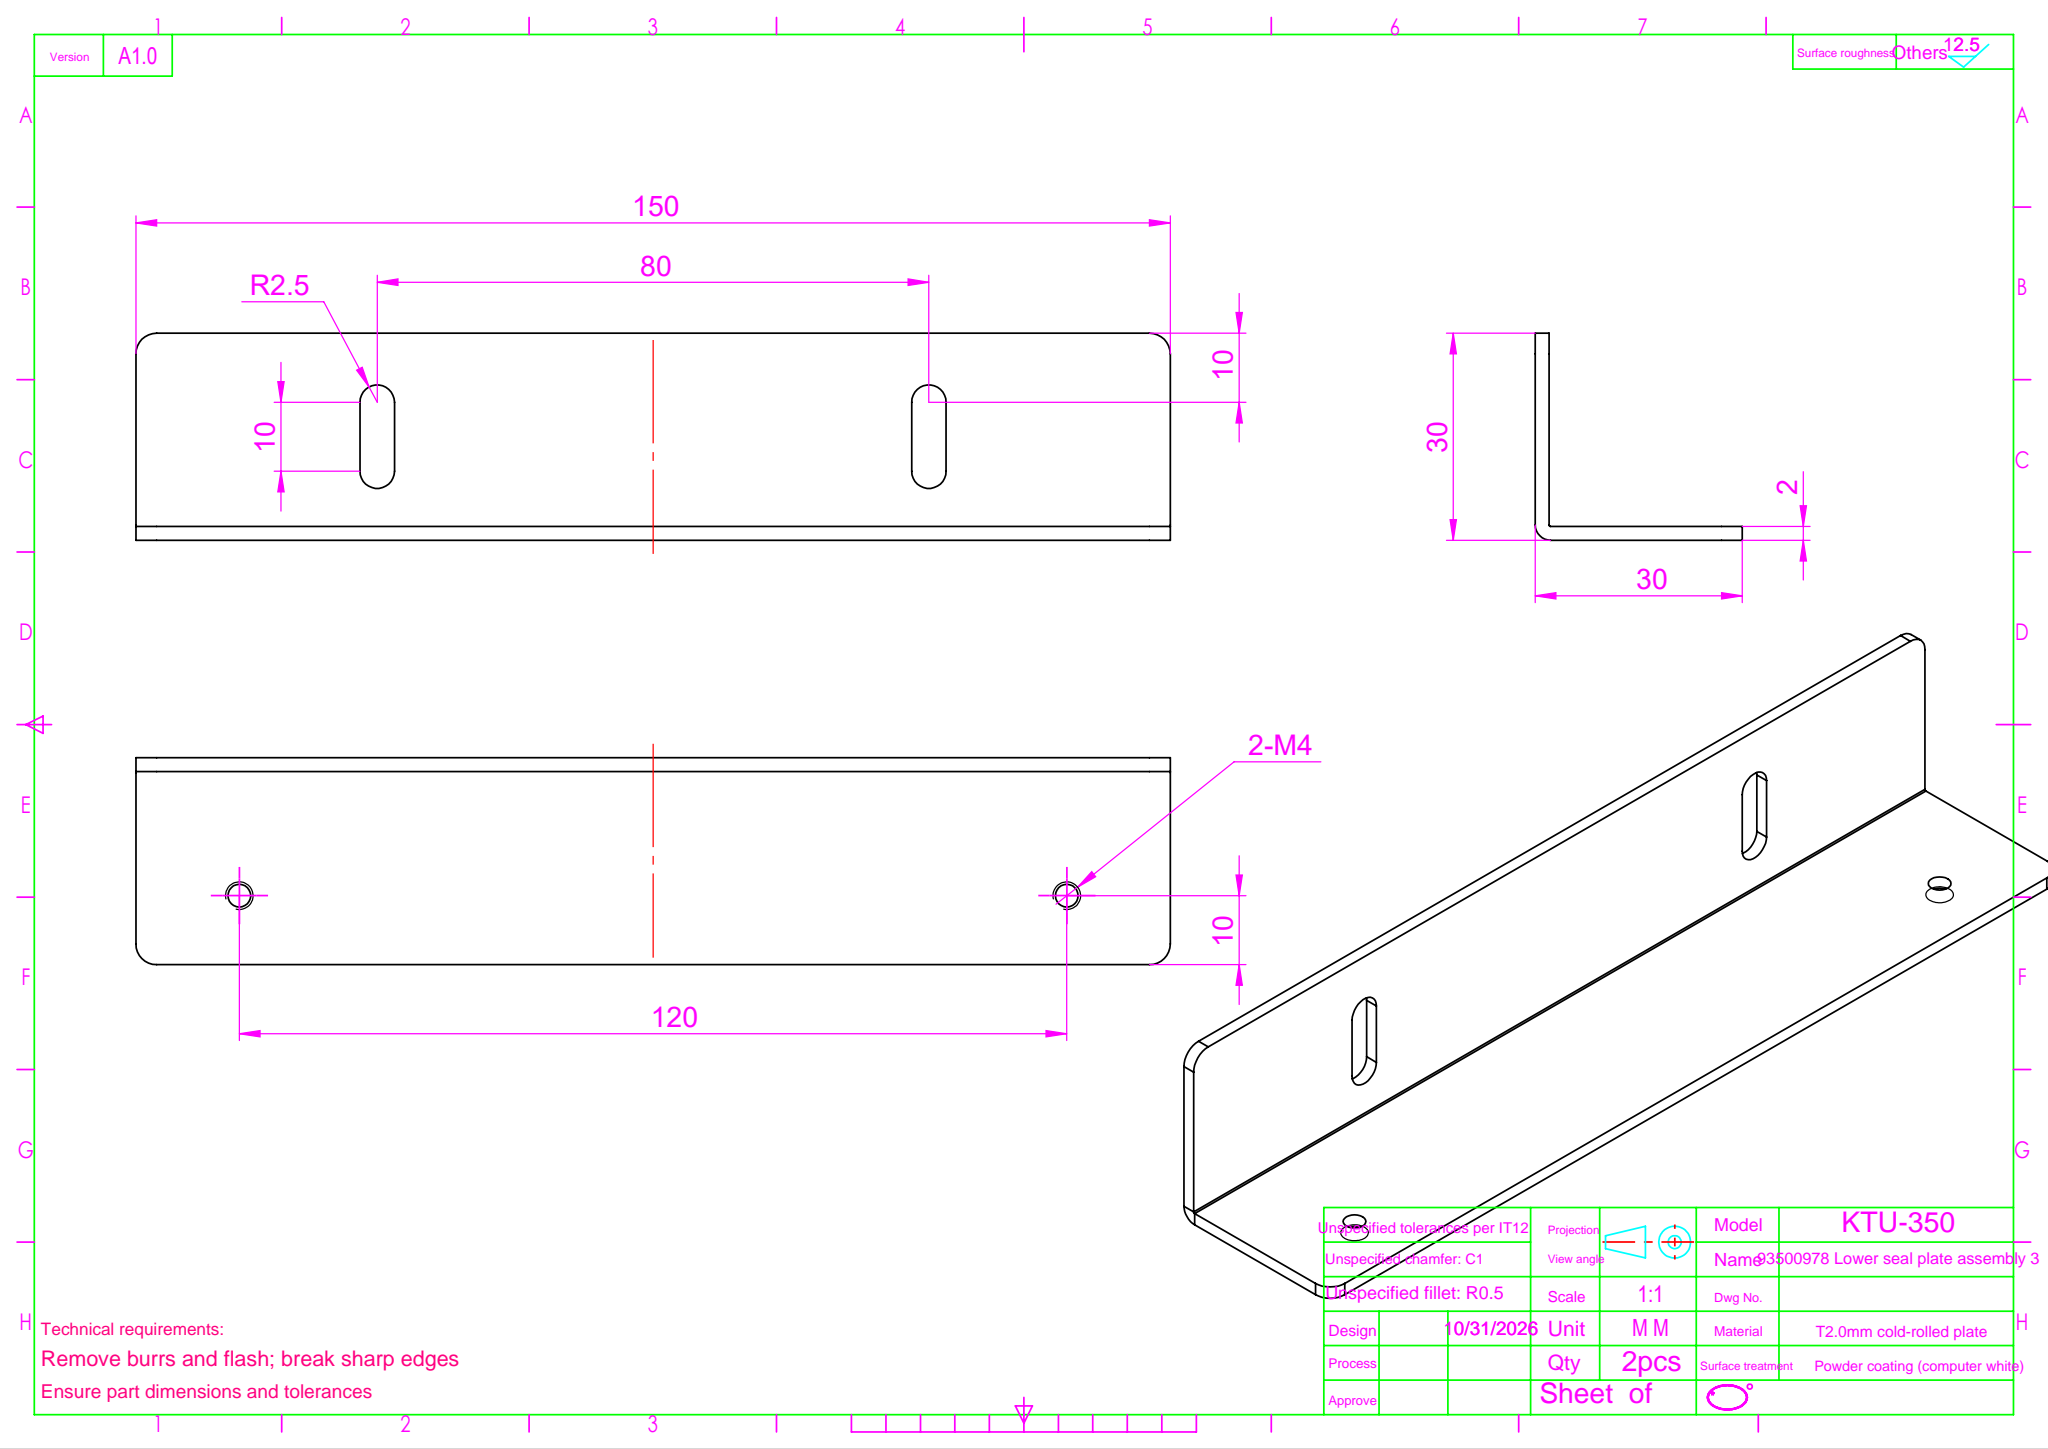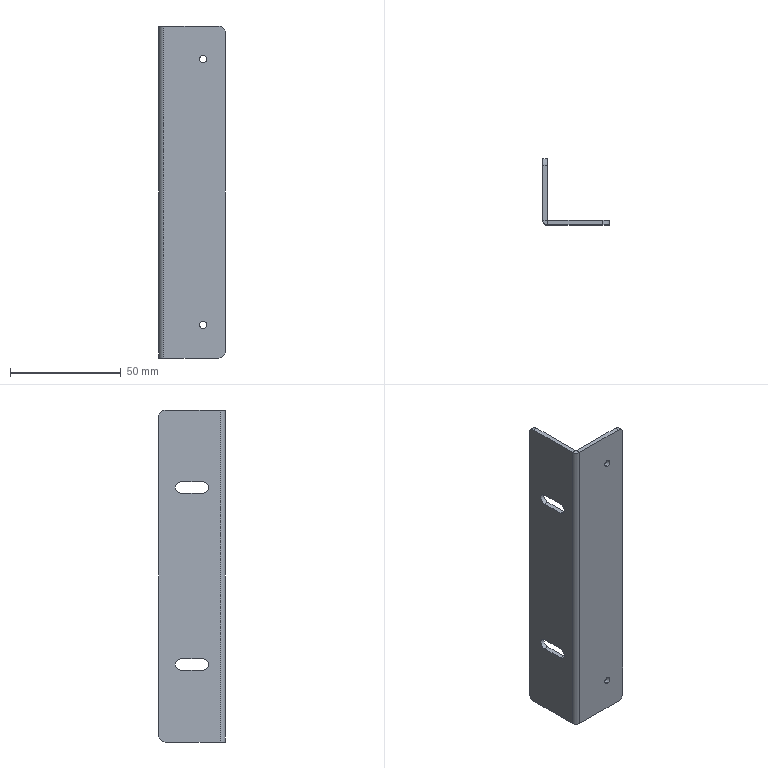Part | SolidWorks | features Fillet 1, FlatPattern 1, HoleWzd 1, ICE 1, SMBaseFlange 1, SheetMetal 1 | 1 solid | 32 faces | box 30 x 30 x 150 mm | volume 16917 mm3 | cylinder 16 | plane 16 | commonest cylinder face diameters 5 x6 3.3 x4 6 x4 0.4 x1 4.4 x1
STEP:
#1=CARTESIAN_POINT('',(5.,2.,61.65));
#2=VERTEX_POINT('',#1);
#3=CARTESIAN_POINT('',(5.,2.,58.35));
#4=VERTEX_POINT('',#3);
#5=CARTESIAN_POINT('',(5.,2.,60.));
#6=DIRECTION('',(0.,-1.,0.));
#7=DIRECTION('',(0.,0.,-1.));
#8=AXIS2_PLACEMENT_3D('',#5,#6,#7);
#9=CIRCLE('',#8,1.65);
#10=EDGE_CURVE('',#2,#4,#9,.T.);
#11=ORIENTED_EDGE('',*,*,#10,.F.);
#12=CARTESIAN_POINT('',(5.,0.,61.65));
#13=VERTEX_POINT('',#12);
#14=CARTESIAN_POINT('',(5.,0.,61.65));
#15=DIRECTION('',(0.,-1.,0.));
#16=VECTOR('',#15,1000.);
#17=LINE('',#14,#16);
#18=EDGE_CURVE('',#2,#13,#17,.T.);
#19=ORIENTED_EDGE('',*,*,#18,.T.);
#20=CARTESIAN_POINT('',(5.,0.,58.35));
#21=VERTEX_POINT('',#20);
#22=CARTESIAN_POINT('',(5.,0.,60.));
#23=DIRECTION('',(0.,-1.,0.));
#24=DIRECTION('',(0.,0.,-1.));
#25=AXIS2_PLACEMENT_3D('',#22,#23,#24);
#26=CIRCLE('',#25,1.65);
#27=EDGE_CURVE('',#13,#21,#26,.T.);
#28=ORIENTED_EDGE('',*,*,#27,.T.);
#29=CARTESIAN_POINT('',(5.,0.,58.35));
#30=DIRECTION('',(0.,-1.,0.));
#31=VECTOR('',#30,1000.);
#32=LINE('',#29,#31);
#33=EDGE_CURVE('',#4,#21,#32,.T.);
#34=ORIENTED_EDGE('',*,*,#33,.F.);
#35=EDGE_LOOP('',(#11,#19,#28,#34));
#36=FACE_OUTER_BOUND('',#35,.T.);
#37=CARTESIAN_POINT('',(5.,0.,60.));
#38=DIRECTION('',(0.,-1.,0.));
#39=DIRECTION('',(0.,0.,-1.));
#40=AXIS2_PLACEMENT_3D('',#37,#38,#39);
#41=CYLINDRICAL_SURFACE('',#40,1.65);
#42=ADVANCED_FACE('',(#36),#41,.F.);
#43=CARTESIAN_POINT('',(5.,2.,-58.35));
#44=VERTEX_POINT('',#43);
#45=CARTESIAN_POINT('',(5.,2.,-61.65));
#46=VERTEX_POINT('',#45);
#47=CARTESIAN_POINT('',(5.,2.,-60.));
#48=DIRECTION('',(0.,-1.,0.));
#49=DIRECTION('',(0.,0.,-1.));
#50=AXIS2_PLACEMENT_3D('',#47,#48,#49);
#51=CIRCLE('',#50,1.65);
#52=EDGE_CURVE('',#44,#46,#51,.T.);
#53=ORIENTED_EDGE('',*,*,#52,.F.);
#54=CARTESIAN_POINT('',(5.,0.,-58.35));
#55=VERTEX_POINT('',#54);
#56=CARTESIAN_POINT('',(5.,0.,-58.35));
#57=DIRECTION('',(0.,-1.,0.));
#58=VECTOR('',#57,1000.);
#59=LINE('',#56,#58);
#60=EDGE_CURVE('',#44,#55,#59,.T.);
#61=ORIENTED_EDGE('',*,*,#60,.T.);
#62=CARTESIAN_POINT('',(5.,0.,-61.65));
#63=VERTEX_POINT('',#62);
#64=CARTESIAN_POINT('',(5.,0.,-60.));
#65=DIRECTION('',(0.,-1.,0.));
#66=DIRECTION('',(0.,0.,-1.));
#67=AXIS2_PLACEMENT_3D('',#64,#65,#66);
#68=CIRCLE('',#67,1.65);
#69=EDGE_CURVE('',#55,#63,#68,.T.);
#70=ORIENTED_EDGE('',*,*,#69,.T.);
#71=CARTESIAN_POINT('',(5.,0.,-61.65));
#72=DIRECTION('',(0.,-1.,0.));
#73=VECTOR('',#72,1000.);
#74=LINE('',#71,#73);
#75=EDGE_CURVE('',#46,#63,#74,.T.);
#76=ORIENTED_EDGE('',*,*,#75,.F.);
#77=EDGE_LOOP('',(#53,#61,#70,#76));
#78=FACE_OUTER_BOUND('',#77,.T.);
#79=CARTESIAN_POINT('',(5.,0.,-60.));
#80=DIRECTION('',(0.,-1.,0.));
#81=DIRECTION('',(0.,0.,-1.));
#82=AXIS2_PLACEMENT_3D('',#79,#80,#81);
#83=CYLINDRICAL_SURFACE('',#82,1.65);
#84=ADVANCED_FACE('',(#78),#83,.F.);
#85=CARTESIAN_POINT('',(-13.,7.5,40.));
#86=VERTEX_POINT('',#85);
#87=CARTESIAN_POINT('',(-13.,10.,42.5));
#88=VERTEX_POINT('',#87);
#89=CARTESIAN_POINT('',(-13.,10.,40.));
#90=DIRECTION('',(-1.,0.,0.));
#91=DIRECTION('',(0.,-1.,0.));
#92=AXIS2_PLACEMENT_3D('',#89,#90,#91);
#93=CIRCLE('',#92,2.5);
#94=EDGE_CURVE('',#86,#88,#93,.T.);
#95=ORIENTED_EDGE('',*,*,#94,.F.);
#96=CARTESIAN_POINT('',(-15.,7.5,40.));
#97=VERTEX_POINT('',#96);
#98=CARTESIAN_POINT('',(-13.,7.5,40.));
#99=DIRECTION('',(-1.,0.,0.));
#100=VECTOR('',#99,1000.);
#101=LINE('',#98,#100);
#102=EDGE_CURVE('',#86,#97,#101,.T.);
#103=ORIENTED_EDGE('',*,*,#102,.T.);
#104=CARTESIAN_POINT('',(-15.,10.,42.5));
#105=VERTEX_POINT('',#104);
#106=CARTESIAN_POINT('',(-15.,10.,40.));
#107=DIRECTION('',(-1.,0.,0.));
#108=DIRECTION('',(0.,-1.,0.));
#109=AXIS2_PLACEMENT_3D('',#106,#107,#108);
#110=CIRCLE('',#109,2.5);
#111=EDGE_CURVE('',#97,#105,#110,.T.);
#112=ORIENTED_EDGE('',*,*,#111,.T.);
#113=CARTESIAN_POINT('',(-13.,10.,42.5));
#114=DIRECTION('',(-1.,0.,0.));
#115=VECTOR('',#114,1000.);
#116=LINE('',#113,#115);
#117=EDGE_CURVE('',#88,#105,#116,.T.);
#118=ORIENTED_EDGE('',*,*,#117,.F.);
#119=EDGE_LOOP('',(#95,#103,#112,#118));
#120=FACE_OUTER_BOUND('',#119,.T.);
#121=CARTESIAN_POINT('',(-13.,10.,40.));
#122=DIRECTION('',(-1.,0.,0.));
#123=DIRECTION('',(0.,-1.,0.));
#124=AXIS2_PLACEMENT_3D('',#121,#122,#123);
#125=CYLINDRICAL_SURFACE('',#124,2.5);
#126=ADVANCED_FACE('',(#120),#125,.F.);
#127=CARTESIAN_POINT('',(-13.,7.5,-40.));
#128=VERTEX_POINT('',#127);
#129=CARTESIAN_POINT('',(-13.,10.,-37.5));
#130=VERTEX_POINT('',#129);
#131=CARTESIAN_POINT('',(-13.,10.,-40.));
#132=DIRECTION('',(-1.,0.,0.));
#133=DIRECTION('',(0.,-1.,0.));
#134=AXIS2_PLACEMENT_3D('',#131,#132,#133);
#135=CIRCLE('',#134,2.5);
#136=EDGE_CURVE('',#128,#130,#135,.T.);
#137=ORIENTED_EDGE('',*,*,#136,.F.);
#138=CARTESIAN_POINT('',(-15.,7.5,-40.));
#139=VERTEX_POINT('',#138);
#140=CARTESIAN_POINT('',(-13.,7.5,-40.));
#141=DIRECTION('',(-1.,0.,0.));
#142=VECTOR('',#141,1000.);
#143=LINE('',#140,#142);
#144=EDGE_CURVE('',#128,#139,#143,.T.);
#145=ORIENTED_EDGE('',*,*,#144,.T.);
#146=CARTESIAN_POINT('',(-15.,10.,-37.5));
#147=VERTEX_POINT('',#146);
#148=CARTESIAN_POINT('',(-15.,10.,-40.));
#149=DIRECTION('',(-1.,0.,0.));
#150=DIRECTION('',(0.,-1.,0.));
#151=AXIS2_PLACEMENT_3D('',#148,#149,#150);
#152=CIRCLE('',#151,2.5);
#153=EDGE_CURVE('',#139,#147,#152,.T.);
#154=ORIENTED_EDGE('',*,*,#153,.T.);
#155=CARTESIAN_POINT('',(-13.,10.,-37.5));
#156=DIRECTION('',(-1.,0.,0.));
#157=VECTOR('',#156,1000.);
#158=LINE('',#155,#157);
#159=EDGE_CURVE('',#130,#147,#158,.T.);
#160=ORIENTED_EDGE('',*,*,#159,.F.);
#161=EDGE_LOOP('',(#137,#145,#154,#160));
#162=FACE_OUTER_BOUND('',#161,.T.);
#163=CARTESIAN_POINT('',(-13.,10.,-40.));
#164=DIRECTION('',(-1.,0.,0.));
#165=DIRECTION('',(0.,-1.,0.));
#166=AXIS2_PLACEMENT_3D('',#163,#164,#165);
#167=CYLINDRICAL_SURFACE('',#166,2.5);
#168=ADVANCED_FACE('',(#162),#167,.F.);
#169=CARTESIAN_POINT('',(-12.8,0.,-75.));
#170=VERTEX_POINT('',#169);
#171=CARTESIAN_POINT('',(-12.8,2.,-75.));
#172=VERTEX_POINT('',#171);
#173=CARTESIAN_POINT('',(-12.8,0.,-75.));
#174=DIRECTION('',(0.,1.,0.));
#175=VECTOR('',#174,1000.);
#176=LINE('',#173,#175);
#177=EDGE_CURVE('',#170,#172,#176,.T.);
#178=ORIENTED_EDGE('',*,*,#177,.F.);
#179=CARTESIAN_POINT('',(-15.,2.2,-75.));
#180=VERTEX_POINT('',#179);
#181=CARTESIAN_POINT('',(-12.8,2.2,-75.));
#182=DIRECTION('',(0.,0.,1.));
#183=DIRECTION('',(-1.,0.,0.));
#184=AXIS2_PLACEMENT_3D('',#181,#182,#183);
#185=CIRCLE('',#184,2.2);
#186=EDGE_CURVE('',#180,#170,#185,.T.);
#187=ORIENTED_EDGE('',*,*,#186,.F.);
#188=CARTESIAN_POINT('',(-13.,2.2,-75.));
#189=VERTEX_POINT('',#188);
#190=CARTESIAN_POINT('',(-13.,2.2,-75.));
#191=DIRECTION('',(-1.,0.,0.));
#192=VECTOR('',#191,1000.);
#193=LINE('',#190,#192);
#194=EDGE_CURVE('',#189,#180,#193,.T.);
#195=ORIENTED_EDGE('',*,*,#194,.F.);
#196=CARTESIAN_POINT('',(-12.8,2.2,-75.));
#197=DIRECTION('',(0.,0.,1.));
#198=DIRECTION('',(1.,0.,0.));
#199=AXIS2_PLACEMENT_3D('',#196,#197,#198);
#200=CIRCLE('',#199,0.2);
#201=EDGE_CURVE('',#189,#172,#200,.T.);
#202=ORIENTED_EDGE('',*,*,#201,.T.);
#203=EDGE_LOOP('',(#178,#187,#195,#202));
#204=FACE_OUTER_BOUND('',#203,.T.);
#205=CARTESIAN_POINT('',(-12.8,0.,-75.));
#206=DIRECTION('',(0.,0.,-1.));
#207=DIRECTION('',(-1.,0.,0.));
#208=AXIS2_PLACEMENT_3D('',#205,#206,#207);
#209=PLANE('',#208);
#210=ADVANCED_FACE('',(#204),#209,.T.);
#211=CARTESIAN_POINT('',(12.,2.,-75.));
#212=VERTEX_POINT('',#211);
#213=CARTESIAN_POINT('',(-15.,2.,-75.));
#214=DIRECTION('',(1.,0.,0.));
#215=VECTOR('',#214,1000.);
#216=LINE('',#213,#215);
#217=EDGE_CURVE('',#172,#212,#216,.T.);
#218=ORIENTED_EDGE('',*,*,#217,.T.);
#219=CARTESIAN_POINT('',(12.,0.,-75.));
#220=VERTEX_POINT('',#219);
#221=CARTESIAN_POINT('',(12.,0.,-75.));
#222=DIRECTION('',(0.,-1.,0.));
#223=VECTOR('',#222,1000.);
#224=LINE('',#221,#223);
#225=EDGE_CURVE('',#212,#220,#224,.T.);
#226=ORIENTED_EDGE('',*,*,#225,.T.);
#227=CARTESIAN_POINT('',(-15.,0.,-75.));
#228=DIRECTION('',(1.,0.,0.));
#229=VECTOR('',#228,1000.);
#230=LINE('',#227,#229);
#231=EDGE_CURVE('',#170,#220,#230,.T.);
#232=ORIENTED_EDGE('',*,*,#231,.F.);
#233=ORIENTED_EDGE('',*,*,#177,.T.);
#234=EDGE_LOOP('',(#218,#226,#232,#233));
#235=FACE_OUTER_BOUND('',#234,.T.);
#236=CARTESIAN_POINT('',(-13.,2.2,-75.));
#237=DIRECTION('',(0.,0.,-1.));
#238=DIRECTION('',(-1.,0.,0.));
#239=AXIS2_PLACEMENT_3D('',#236,#237,#238);
#240=PLANE('',#239);
#241=ADVANCED_FACE('',(#235),#240,.T.);
#242=CARTESIAN_POINT('',(-15.,2.2,75.));
#243=VERTEX_POINT('',#242);
#244=CARTESIAN_POINT('',(-13.,2.2,75.));
#245=VERTEX_POINT('',#244);
#246=CARTESIAN_POINT('',(-15.,2.2,75.));
#247=DIRECTION('',(1.,0.,0.));
#248=VECTOR('',#247,1000.);
#249=LINE('',#246,#248);
#250=EDGE_CURVE('',#243,#245,#249,.T.);
#251=ORIENTED_EDGE('',*,*,#250,.F.);
#252=CARTESIAN_POINT('',(-12.8,0.,75.));
#253=VERTEX_POINT('',#252);
#254=CARTESIAN_POINT('',(-12.8,2.2,75.));
#255=DIRECTION('',(0.,0.,1.));
#256=DIRECTION('',(-1.,0.,0.));
#257=AXIS2_PLACEMENT_3D('',#254,#255,#256);
#258=CIRCLE('',#257,2.2);
#259=EDGE_CURVE('',#243,#253,#258,.T.);
#260=ORIENTED_EDGE('',*,*,#259,.T.);
#261=CARTESIAN_POINT('',(-12.8,2.,75.));
#262=VERTEX_POINT('',#261);
#263=CARTESIAN_POINT('',(-12.8,2.,75.));
#264=DIRECTION('',(0.,-1.,0.));
#265=VECTOR('',#264,1000.);
#266=LINE('',#263,#265);
#267=EDGE_CURVE('',#262,#253,#266,.T.);
#268=ORIENTED_EDGE('',*,*,#267,.F.);
#269=CARTESIAN_POINT('',(-12.8,2.2,75.));
#270=DIRECTION('',(0.,0.,1.));
#271=DIRECTION('',(1.,0.,0.));
#272=AXIS2_PLACEMENT_3D('',#269,#270,#271);
#273=CIRCLE('',#272,0.2);
#274=EDGE_CURVE('',#245,#262,#273,.T.);
#275=ORIENTED_EDGE('',*,*,#274,.F.);
#276=EDGE_LOOP('',(#251,#260,#268,#275));
#277=FACE_OUTER_BOUND('',#276,.T.);
#278=CARTESIAN_POINT('',(-15.,2.2,75.));
#279=DIRECTION('',(0.,0.,1.));
#280=DIRECTION('',(1.,0.,0.));
#281=AXIS2_PLACEMENT_3D('',#278,#279,#280);
#282=PLANE('',#281);
#283=ADVANCED_FACE('',(#277),#282,.T.);
#284=CARTESIAN_POINT('',(-13.,27.,75.));
#285=VERTEX_POINT('',#284);
#286=CARTESIAN_POINT('',(-13.,30.,75.));
#287=DIRECTION('',(0.,-1.,0.));
#288=VECTOR('',#287,1000.);
#289=LINE('',#286,#288);
#290=EDGE_CURVE('',#285,#245,#289,.T.);
#291=ORIENTED_EDGE('',*,*,#290,.F.);
#292=CARTESIAN_POINT('',(-15.,27.,75.));
#293=VERTEX_POINT('',#292);
#294=CARTESIAN_POINT('',(-15.,27.,75.));
#295=DIRECTION('',(-1.,0.,0.));
#296=VECTOR('',#295,1000.);
#297=LINE('',#294,#296);
#298=EDGE_CURVE('',#285,#293,#297,.T.);
#299=ORIENTED_EDGE('',*,*,#298,.T.);
#300=CARTESIAN_POINT('',(-15.,30.,75.));
#301=DIRECTION('',(0.,-1.,0.));
#302=VECTOR('',#301,1000.);
#303=LINE('',#300,#302);
#304=EDGE_CURVE('',#293,#243,#303,.T.);
#305=ORIENTED_EDGE('',*,*,#304,.T.);
#306=ORIENTED_EDGE('',*,*,#250,.T.);
#307=EDGE_LOOP('',(#291,#299,#305,#306));
#308=FACE_OUTER_BOUND('',#307,.T.);
#309=CARTESIAN_POINT('',(-12.8,2.,75.));
#310=DIRECTION('',(0.,0.,1.));
#311=DIRECTION('',(1.,0.,0.));
#312=AXIS2_PLACEMENT_3D('',#309,#310,#311);
#313=PLANE('',#312);
#314=ADVANCED_FACE('',(#308),#313,.T.);
#315=CARTESIAN_POINT('',(5.,0.,60.));
#316=DIRECTION('',(0.,-1.,0.));
#317=DIRECTION('',(0.,0.,-1.));
#318=AXIS2_PLACEMENT_3D('',#315,#316,#317);
#319=CIRCLE('',#318,1.65);
#320=EDGE_CURVE('',#21,#13,#319,.T.);
#321=ORIENTED_EDGE('',*,*,#320,.F.);
#322=ORIENTED_EDGE('',*,*,#27,.F.);
#323=EDGE_LOOP('',(#321,#322));
#324=FACE_BOUND('',#323,.T.);
#325=CARTESIAN_POINT('',(5.,0.,-60.));
#326=DIRECTION('',(0.,-1.,0.));
#327=DIRECTION('',(0.,0.,-1.));
#328=AXIS2_PLACEMENT_3D('',#325,#326,#327);
#329=CIRCLE('',#328,1.65);
#330=EDGE_CURVE('',#63,#55,#329,.T.);
#331=ORIENTED_EDGE('',*,*,#330,.F.);
#332=ORIENTED_EDGE('',*,*,#69,.F.);
#333=EDGE_LOOP('',(#331,#332));
#334=FACE_BOUND('',#333,.T.);
#335=ORIENTED_EDGE('',*,*,#231,.T.);
#336=CARTESIAN_POINT('',(15.,0.,-72.));
#337=VERTEX_POINT('',#336);
#338=CARTESIAN_POINT('',(12.,0.,-72.));
#339=DIRECTION('',(0.,-1.,0.));
#340=DIRECTION('',(0.,0.,-1.));
#341=AXIS2_PLACEMENT_3D('',#338,#339,#340);
#342=CIRCLE('',#341,3.);
#343=EDGE_CURVE('',#220,#337,#342,.T.);
#344=ORIENTED_EDGE('',*,*,#343,.T.);
#345=CARTESIAN_POINT('',(15.,0.,72.));
#346=VERTEX_POINT('',#345);
#347=CARTESIAN_POINT('',(15.,0.,-75.));
#348=DIRECTION('',(0.,0.,1.));
#349=VECTOR('',#348,1000.);
#350=LINE('',#347,#349);
#351=EDGE_CURVE('',#337,#346,#350,.T.);
#352=ORIENTED_EDGE('',*,*,#351,.T.);
#353=CARTESIAN_POINT('',(12.,0.,75.));
#354=VERTEX_POINT('',#353);
#355=CARTESIAN_POINT('',(12.,0.,72.));
#356=DIRECTION('',(0.,-1.,0.));
#357=DIRECTION('',(0.,0.,-1.));
#358=AXIS2_PLACEMENT_3D('',#355,#356,#357);
#359=CIRCLE('',#358,3.);
#360=EDGE_CURVE('',#346,#354,#359,.T.);
#361=ORIENTED_EDGE('',*,*,#360,.T.);
#362=CARTESIAN_POINT('',(-15.,0.,75.));
#363=DIRECTION('',(1.,0.,0.));
#364=VECTOR('',#363,1000.);
#365=LINE('',#362,#364);
#366=EDGE_CURVE('',#253,#354,#365,.T.);
#367=ORIENTED_EDGE('',*,*,#366,.F.);
#368=CARTESIAN_POINT('',(-12.8,0.,-75.));
#369=DIRECTION('',(0.,0.,1.));
#370=VECTOR('',#369,1000.);
#371=LINE('',#368,#370);
#372=EDGE_CURVE('',#170,#253,#371,.T.);
#373=ORIENTED_EDGE('',*,*,#372,.F.);
#374=EDGE_LOOP('',(#335,#344,#352,#361,#367,#373));
#375=FACE_OUTER_BOUND('',#374,.T.);
#376=CARTESIAN_POINT('',(-15.,0.,-75.));
#377=DIRECTION('',(0.,-1.,0.));
#378=DIRECTION('',(0.,0.,-1.));
#379=AXIS2_PLACEMENT_3D('',#376,#377,#378);
#380=PLANE('',#379);
#381=ADVANCED_FACE('',(#324,#334,#375),#380,.T.);
#382=ORIENTED_EDGE('',*,*,#259,.F.);
#383=CARTESIAN_POINT('',(-15.,2.2,-75.));
#384=DIRECTION('',(0.,0.,1.));
#385=VECTOR('',#384,1000.);
#386=LINE('',#383,#385);
#387=EDGE_CURVE('',#180,#243,#386,.T.);
#388=ORIENTED_EDGE('',*,*,#387,.F.);
#389=ORIENTED_EDGE('',*,*,#186,.T.);
#390=ORIENTED_EDGE('',*,*,#372,.T.);
#391=EDGE_LOOP('',(#382,#388,#389,#390));
#392=FACE_OUTER_BOUND('',#391,.T.);
#393=CARTESIAN_POINT('',(-12.8,2.2,-75.));
#394=DIRECTION('',(0.,0.,1.));
#395=DIRECTION('',(1.,0.,0.));
#396=AXIS2_PLACEMENT_3D('',#393,#394,#395);
#397=CYLINDRICAL_SURFACE('',#396,2.2);
#398=ADVANCED_FACE('',(#392),#397,.T.);
#399=CARTESIAN_POINT('',(-15.,20.,42.5));
#400=VERTEX_POINT('',#399);
#401=CARTESIAN_POINT('',(-15.,20.,37.5));
#402=VERTEX_POINT('',#401);
#403=CARTESIAN_POINT('',(-15.,20.,40.));
#404=DIRECTION('',(-1.,0.,0.));
#405=DIRECTION('',(0.,-1.,0.));
#406=AXIS2_PLACEMENT_3D('',#403,#404,#405);
#407=CIRCLE('',#406,2.5);
#408=EDGE_CURVE('',#400,#402,#407,.T.);
#409=ORIENTED_EDGE('',*,*,#408,.F.);
#410=CARTESIAN_POINT('',(-15.,20.,42.5));
#411=DIRECTION('',(0.,1.,0.));
#412=VECTOR('',#411,1000.);
#413=LINE('',#410,#412);
#414=EDGE_CURVE('',#105,#400,#413,.T.);
#415=ORIENTED_EDGE('',*,*,#414,.F.);
#416=ORIENTED_EDGE('',*,*,#111,.F.);
#417=CARTESIAN_POINT('',(-15.,10.,37.5));
#418=VERTEX_POINT('',#417);
#419=CARTESIAN_POINT('',(-15.,10.,40.));
#420=DIRECTION('',(-1.,0.,0.));
#421=DIRECTION('',(0.,-1.,0.));
#422=AXIS2_PLACEMENT_3D('',#419,#420,#421);
#423=CIRCLE('',#422,2.5);
#424=EDGE_CURVE('',#418,#97,#423,.T.);
#425=ORIENTED_EDGE('',*,*,#424,.F.);
#426=CARTESIAN_POINT('',(-15.,20.,37.5));
#427=DIRECTION('',(0.,-1.,0.));
#428=VECTOR('',#427,1000.);
#429=LINE('',#426,#428);
#430=EDGE_CURVE('',#402,#418,#429,.T.);
#431=ORIENTED_EDGE('',*,*,#430,.F.);
#432=EDGE_LOOP('',(#409,#415,#416,#425,#431));
#433=FACE_BOUND('',#432,.T.);
#434=CARTESIAN_POINT('',(-15.,20.,-37.5));
#435=VERTEX_POINT('',#434);
#436=CARTESIAN_POINT('',(-15.,20.,-42.5));
#437=VERTEX_POINT('',#436);
#438=CARTESIAN_POINT('',(-15.,20.,-40.));
#439=DIRECTION('',(-1.,0.,0.));
#440=DIRECTION('',(0.,-1.,0.));
#441=AXIS2_PLACEMENT_3D('',#438,#439,#440);
#442=CIRCLE('',#441,2.5);
#443=EDGE_CURVE('',#435,#437,#442,.T.);
#444=ORIENTED_EDGE('',*,*,#443,.F.);
#445=CARTESIAN_POINT('',(-15.,20.,-37.5));
#446=DIRECTION('',(0.,1.,0.));
#447=VECTOR('',#446,1000.);
#448=LINE('',#445,#447);
#449=EDGE_CURVE('',#147,#435,#448,.T.);
#450=ORIENTED_EDGE('',*,*,#449,.F.);
#451=ORIENTED_EDGE('',*,*,#153,.F.);
#452=CARTESIAN_POINT('',(-15.,10.,-42.5));
#453=VERTEX_POINT('',#452);
#454=CARTESIAN_POINT('',(-15.,10.,-40.));
#455=DIRECTION('',(-1.,0.,0.));
#456=DIRECTION('',(0.,-1.,0.));
#457=AXIS2_PLACEMENT_3D('',#454,#455,#456);
#458=CIRCLE('',#457,2.5);
#459=EDGE_CURVE('',#453,#139,#458,.T.);
#460=ORIENTED_EDGE('',*,*,#459,.F.);
#461=CARTESIAN_POINT('',(-15.,20.,-42.5));
#462=DIRECTION('',(0.,-1.,0.));
#463=VECTOR('',#462,1000.);
#464=LINE('',#461,#463);
#465=EDGE_CURVE('',#437,#453,#464,.T.);
#466=ORIENTED_EDGE('',*,*,#465,.F.);
#467=EDGE_LOOP('',(#444,#450,#451,#460,#466));
#468=FACE_BOUND('',#467,.T.);
#469=CARTESIAN_POINT('',(-15.,30.,-72.));
#470=VERTEX_POINT('',#469);
#471=CARTESIAN_POINT('',(-15.,30.,72.));
#472=VERTEX_POINT('',#471);
#473=CARTESIAN_POINT('',(-15.,30.,-75.));
#474=DIRECTION('',(0.,0.,1.));
#475=VECTOR('',#474,1000.);
#476=LINE('',#473,#475);
#477=EDGE_CURVE('',#470,#472,#476,.T.);
#478=ORIENTED_EDGE('',*,*,#477,.F.);
#479=CARTESIAN_POINT('',(-15.,27.,-75.));
#480=VERTEX_POINT('',#479);
#481=CARTESIAN_POINT('',(-15.,27.,-72.));
#482=DIRECTION('',(-1.,0.,0.));
#483=DIRECTION('',(0.,-1.,0.));
#484=AXIS2_PLACEMENT_3D('',#481,#482,#483);
#485=CIRCLE('',#484,3.);
#486=EDGE_CURVE('',#470,#480,#485,.T.);
#487=ORIENTED_EDGE('',*,*,#486,.T.);
#488=CARTESIAN_POINT('',(-15.,30.,-75.));
#489=DIRECTION('',(0.,-1.,0.));
#490=VECTOR('',#489,1000.);
#491=LINE('',#488,#490);
#492=EDGE_CURVE('',#480,#180,#491,.T.);
#493=ORIENTED_EDGE('',*,*,#492,.T.);
#494=ORIENTED_EDGE('',*,*,#387,.T.);
#495=ORIENTED_EDGE('',*,*,#304,.F.);
#496=CARTESIAN_POINT('',(-15.,27.,72.));
#497=DIRECTION('',(-1.,0.,0.));
#498=DIRECTION('',(0.,-1.,0.));
#499=AXIS2_PLACEMENT_3D('',#496,#497,#498);
#500=CIRCLE('',#499,3.);
#501=EDGE_CURVE('',#293,#472,#500,.T.);
#502=ORIENTED_EDGE('',*,*,#501,.T.);
#503=EDGE_LOOP('',(#478,#487,#493,#494,#495,#502));
#504=FACE_OUTER_BOUND('',#503,.T.);
#505=CARTESIAN_POINT('',(-15.,30.,-75.));
#506=DIRECTION('',(-1.,0.,0.));
#507=DIRECTION('',(0.,-1.,0.));
#508=AXIS2_PLACEMENT_3D('',#505,#506,#507);
#509=PLANE('',#508);
#510=ADVANCED_FACE('',(#433,#468,#504),#509,.T.);
#511=CARTESIAN_POINT('',(-13.,30.,-72.));
#512=VERTEX_POINT('',#511);
#513=CARTESIAN_POINT('',(-13.,30.,72.));
#514=VERTEX_POINT('',#513);
#515=CARTESIAN_POINT('',(-13.,30.,-75.));
#516=DIRECTION('',(0.,0.,1.));
#517=VECTOR('',#516,1000.);
#518=LINE('',#515,#517);
#519=EDGE_CURVE('',#512,#514,#518,.T.);
#520=ORIENTED_EDGE('',*,*,#519,.F.);
#521=CARTESIAN_POINT('',(-15.,30.,-72.));
#522=DIRECTION('',(-1.,0.,0.));
#523=VECTOR('',#522,1000.);
#524=LINE('',#521,#523);
#525=EDGE_CURVE('',#512,#470,#524,.T.);
#526=ORIENTED_EDGE('',*,*,#525,.T.);
#527=ORIENTED_EDGE('',*,*,#477,.T.);
#528=CARTESIAN_POINT('',(-13.,30.,72.));
#529=DIRECTION('',(1.,0.,0.));
#530=VECTOR('',#529,1000.);
#531=LINE('',#528,#530);
#532=EDGE_CURVE('',#472,#514,#531,.T.);
#533=ORIENTED_EDGE('',*,*,#532,.T.);
#534=EDGE_LOOP('',(#520,#526,#527,#533));
#535=FACE_OUTER_BOUND('',#534,.T.);
#536=CARTESIAN_POINT('',(-15.,30.,-75.));
#537=DIRECTION('',(0.,-1.,0.));
#538=DIRECTION('',(0.,0.,-1.));
#539=AXIS2_PLACEMENT_3D('',#536,#537,#538);
#540=PLANE('',#539);
#541=ADVANCED_FACE('',(#535),#540,.F.);
#542=CARTESIAN_POINT('',(-13.,20.,42.5));
#543=VERTEX_POINT('',#542);
#544=CARTESIAN_POINT('',(-13.,20.,42.5));
#545=DIRECTION('',(0.,1.,0.));
#546=VECTOR('',#545,1000.);
#547=LINE('',#544,#546);
#548=EDGE_CURVE('',#88,#543,#547,.T.);
#549=ORIENTED_EDGE('',*,*,#548,.T.);
#550=CARTESIAN_POINT('',(-13.,20.,37.5));
#551=VERTEX_POINT('',#550);
#552=CARTESIAN_POINT('',(-13.,20.,40.));
#553=DIRECTION('',(-1.,0.,0.));
#554=DIRECTION('',(0.,-1.,0.));
#555=AXIS2_PLACEMENT_3D('',#552,#553,#554);
#556=CIRCLE('',#555,2.5);
#557=EDGE_CURVE('',#543,#551,#556,.T.);
#558=ORIENTED_EDGE('',*,*,#557,.T.);
#559=CARTESIAN_POINT('',(-13.,10.,37.5));
#560=VERTEX_POINT('',#559);
#561=CARTESIAN_POINT('',(-13.,20.,37.5));
#562=DIRECTION('',(0.,-1.,0.));
#563=VECTOR('',#562,1000.);
#564=LINE('',#561,#563);
#565=EDGE_CURVE('',#551,#560,#564,.T.);
#566=ORIENTED_EDGE('',*,*,#565,.T.);
#567=CARTESIAN_POINT('',(-13.,10.,40.));
#568=DIRECTION('',(-1.,0.,0.));
#569=DIRECTION('',(0.,-1.,0.));
#570=AXIS2_PLACEMENT_3D('',#567,#568,#569);
#571=CIRCLE('',#570,2.5);
#572=EDGE_CURVE('',#560,#86,#571,.T.);
#573=ORIENTED_EDGE('',*,*,#572,.T.);
#574=ORIENTED_EDGE('',*,*,#94,.T.);
#575=EDGE_LOOP('',(#549,#558,#566,#573,#574));
#576=FACE_BOUND('',#575,.T.);
#577=CARTESIAN_POINT('',(-13.,20.,-37.5));
#578=VERTEX_POINT('',#577);
#579=CARTESIAN_POINT('',(-13.,20.,-37.5));
#580=DIRECTION('',(0.,1.,0.));
#581=VECTOR('',#580,1000.);
#582=LINE('',#579,#581);
#583=EDGE_CURVE('',#130,#578,#582,.T.);
#584=ORIENTED_EDGE('',*,*,#583,.T.);
#585=CARTESIAN_POINT('',(-13.,20.,-42.5));
#586=VERTEX_POINT('',#585);
#587=CARTESIAN_POINT('',(-13.,20.,-40.));
#588=DIRECTION('',(-1.,0.,0.));
#589=DIRECTION('',(0.,-1.,0.));
#590=AXIS2_PLACEMENT_3D('',#587,#588,#589);
#591=CIRCLE('',#590,2.5);
#592=EDGE_CURVE('',#578,#586,#591,.T.);
#593=ORIENTED_EDGE('',*,*,#592,.T.);
#594=CARTESIAN_POINT('',(-13.,10.,-42.5));
#595=VERTEX_POINT('',#594);
#596=CARTESIAN_POINT('',(-13.,20.,-42.5));
#597=DIRECTION('',(0.,-1.,0.));
#598=VECTOR('',#597,1000.);
#599=LINE('',#596,#598);
#600=EDGE_CURVE('',#586,#595,#599,.T.);
#601=ORIENTED_EDGE('',*,*,#600,.T.);
#602=CARTESIAN_POINT('',(-13.,10.,-40.));
#603=DIRECTION('',(-1.,0.,0.));
#604=DIRECTION('',(0.,-1.,0.));
#605=AXIS2_PLACEMENT_3D('',#602,#603,#604);
#606=CIRCLE('',#605,2.5);
#607=EDGE_CURVE('',#595,#128,#606,.T.);
#608=ORIENTED_EDGE('',*,*,#607,.T.);
#609=ORIENTED_EDGE('',*,*,#136,.T.);
#610=EDGE_LOOP('',(#584,#593,#601,#608,#609));
#611=FACE_BOUND('',#610,.T.);
#612=CARTESIAN_POINT('',(-13.,27.,-75.));
#613=VERTEX_POINT('',#612);
#614=CARTESIAN_POINT('',(-13.,30.,-75.));
#615=DIRECTION('',(0.,-1.,0.));
#616=VECTOR('',#615,1000.);
#617=LINE('',#614,#616);
#618=EDGE_CURVE('',#613,#189,#617,.T.);
#619=ORIENTED_EDGE('',*,*,#618,.F.);
#620=CARTESIAN_POINT('',(-13.,27.,-72.));
#621=DIRECTION('',(1.,0.,0.));
#622=DIRECTION('',(0.,-1.,0.));
#623=AXIS2_PLACEMENT_3D('',#620,#621,#622);
#624=CIRCLE('',#623,3.);
#625=EDGE_CURVE('',#613,#512,#624,.T.);
#626=ORIENTED_EDGE('',*,*,#625,.T.);
#627=ORIENTED_EDGE('',*,*,#519,.T.);
#628=CARTESIAN_POINT('',(-13.,27.,72.));
#629=DIRECTION('',(1.,0.,0.));
#630=DIRECTION('',(0.,-1.,0.));
#631=AXIS2_PLACEMENT_3D('',#628,#629,#630);
#632=CIRCLE('',#631,3.);
#633=EDGE_CURVE('',#514,#285,#632,.T.);
#634=ORIENTED_EDGE('',*,*,#633,.T.);
#635=ORIENTED_EDGE('',*,*,#290,.T.);
#636=CARTESIAN_POINT('',(-13.,2.2,-75.));
#637=DIRECTION('',(0.,0.,1.));
#638=VECTOR('',#637,1000.);
#639=LINE('',#636,#638);
#640=EDGE_CURVE('',#189,#245,#639,.T.);
#641=ORIENTED_EDGE('',*,*,#640,.F.);
#642=EDGE_LOOP('',(#619,#626,#627,#634,#635,#641));
#643=FACE_OUTER_BOUND('',#642,.T.);
#644=CARTESIAN_POINT('',(-13.,30.,-75.));
#645=DIRECTION('',(-1.,0.,0.));
#646=DIRECTION('',(0.,-1.,0.));
#647=AXIS2_PLACEMENT_3D('',#644,#645,#646);
#648=PLANE('',#647);
#649=ADVANCED_FACE('',(#576,#611,#643),#648,.F.);
#650=ORIENTED_EDGE('',*,*,#274,.T.);
#651=CARTESIAN_POINT('',(-12.8,2.,-75.));
#652=DIRECTION('',(0.,0.,1.));
#653=VECTOR('',#652,1000.);
#654=LINE('',#651,#653);
#655=EDGE_CURVE('',#172,#262,#654,.T.);
#656=ORIENTED_EDGE('',*,*,#655,.F.);
#657=ORIENTED_EDGE('',*,*,#201,.F.);
#658=ORIENTED_EDGE('',*,*,#640,.T.);
#659=EDGE_LOOP('',(#650,#656,#657,#658));
#660=FACE_OUTER_BOUND('',#659,.T.);
#661=CARTESIAN_POINT('',(-12.8,2.2,-75.));
#662=DIRECTION('',(0.,0.,1.));
#663=DIRECTION('',(1.,0.,0.));
#664=AXIS2_PLACEMENT_3D('',#661,#662,#663);
#665=CYLINDRICAL_SURFACE('',#664,0.2);
#666=ADVANCED_FACE('',(#660),#665,.F.);
#667=CARTESIAN_POINT('',(5.,2.,60.));
#668=DIRECTION('',(0.,-1.,0.));
#669=DIRECTION('',(0.,0.,-1.));
#670=AXIS2_PLACEMENT_3D('',#667,#668,#669);
#671=CIRCLE('',#670,1.65);
#672=EDGE_CURVE('',#4,#2,#671,.T.);
#673=ORIENTED_EDGE('',*,*,#672,.T.);
#674=ORIENTED_EDGE('',*,*,#10,.T.);
#675=EDGE_LOOP('',(#673,#674));
#676=FACE_BOUND('',#675,.T.);
#677=CARTESIAN_POINT('',(5.,2.,-60.));
#678=DIRECTION('',(0.,-1.,0.));
#679=DIRECTION('',(0.,0.,-1.));
#680=AXIS2_PLACEMENT_3D('',#677,#678,#679);
#681=CIRCLE('',#680,1.65);
#682=EDGE_CURVE('',#46,#44,#681,.T.);
#683=ORIENTED_EDGE('',*,*,#682,.T.);
#684=ORIENTED_EDGE('',*,*,#52,.T.);
#685=EDGE_LOOP('',(#683,#684));
#686=FACE_BOUND('',#685,.T.);
#687=CARTESIAN_POINT('',(15.,2.,-72.));
#688=VERTEX_POINT('',#687);
#689=CARTESIAN_POINT('',(15.,2.,72.));
#690=VERTEX_POINT('',#689);
#691=CARTESIAN_POINT('',(15.,2.,-75.));
#692=DIRECTION('',(0.,0.,1.));
#693=VECTOR('',#692,1000.);
#694=LINE('',#691,#693);
#695=EDGE_CURVE('',#688,#690,#694,.T.);
#696=ORIENTED_EDGE('',*,*,#695,.F.);
#697=CARTESIAN_POINT('',(12.,2.,-72.));
#698=DIRECTION('',(0.,1.,0.));
#699=DIRECTION('',(0.,0.,-1.));
#700=AXIS2_PLACEMENT_3D('',#697,#698,#699);
#701=CIRCLE('',#700,3.);
#702=EDGE_CURVE('',#688,#212,#701,.T.);
#703=ORIENTED_EDGE('',*,*,#702,.T.);
#704=ORIENTED_EDGE('',*,*,#217,.F.);
#705=ORIENTED_EDGE('',*,*,#655,.T.);
#706=CARTESIAN_POINT('',(12.,2.,75.));
#707=VERTEX_POINT('',#706);
#708=CARTESIAN_POINT('',(-15.,2.,75.));
#709=DIRECTION('',(1.,0.,0.));
#710=VECTOR('',#709,1000.);
#711=LINE('',#708,#710);
#712=EDGE_CURVE('',#262,#707,#711,.T.);
#713=ORIENTED_EDGE('',*,*,#712,.T.);
#714=CARTESIAN_POINT('',(12.,2.,72.));
#715=DIRECTION('',(0.,1.,0.));
#716=DIRECTION('',(0.,0.,-1.));
#717=AXIS2_PLACEMENT_3D('',#714,#715,#716);
#718=CIRCLE('',#717,3.);
#719=EDGE_CURVE('',#707,#690,#718,.T.);
#720=ORIENTED_EDGE('',*,*,#719,.T.);
#721=EDGE_LOOP('',(#696,#703,#704,#705,#713,#720));
#722=FACE_OUTER_BOUND('',#721,.T.);
#723=CARTESIAN_POINT('',(-15.,2.,-75.));
#724=DIRECTION('',(0.,-1.,0.));
#725=DIRECTION('',(0.,0.,-1.));
#726=AXIS2_PLACEMENT_3D('',#723,#724,#725);
#727=PLANE('',#726);
#728=ADVANCED_FACE('',(#676,#686,#722),#727,.F.);
#729=ORIENTED_EDGE('',*,*,#351,.F.);
#730=CARTESIAN_POINT('',(15.,2.,-72.));
#731=DIRECTION('',(0.,1.,0.));
#732=VECTOR('',#731,1000.);
#733=LINE('',#730,#732);
#734=EDGE_CURVE('',#337,#688,#733,.T.);
#735=ORIENTED_EDGE('',*,*,#734,.T.);
#736=ORIENTED_EDGE('',*,*,#695,.T.);
#737=CARTESIAN_POINT('',(15.,0.,72.));
#738=DIRECTION('',(0.,-1.,0.));
#739=VECTOR('',#738,1000.);
#740=LINE('',#737,#739);
#741=EDGE_CURVE('',#690,#346,#740,.T.);
#742=ORIENTED_EDGE('',*,*,#741,.T.);
#743=EDGE_LOOP('',(#729,#735,#736,#742));
#744=FACE_OUTER_BOUND('',#743,.T.);
#745=CARTESIAN_POINT('',(15.,2.,-75.));
#746=DIRECTION('',(-1.,0.,0.));
#747=DIRECTION('',(0.,0.,1.));
#748=AXIS2_PLACEMENT_3D('',#745,#746,#747);
#749=PLANE('',#748);
#750=ADVANCED_FACE('',(#744),#749,.F.);
#751=ORIENTED_EDGE('',*,*,#492,.F.);
#752=CARTESIAN_POINT('',(-12.8,27.,-75.));
#753=DIRECTION('',(1.,0.,0.));
#754=VECTOR('',#753,1000.);
#755=LINE('',#752,#754);
#756=EDGE_CURVE('',#480,#613,#755,.T.);
#757=ORIENTED_EDGE('',*,*,#756,.T.);
#758=ORIENTED_EDGE('',*,*,#618,.T.);
#759=ORIENTED_EDGE('',*,*,#194,.T.);
#760=EDGE_LOOP('',(#751,#757,#758,#759));
#761=FACE_OUTER_BOUND('',#760,.T.);
#762=CARTESIAN_POINT('',(-12.8,2.2,-75.));
#763=DIRECTION('',(0.,0.,1.));
#764=DIRECTION('',(1.,0.,0.));
#765=AXIS2_PLACEMENT_3D('',#762,#763,#764);
#766=PLANE('',#765);
#767=ADVANCED_FACE('',(#761),#766,.F.);
#768=ORIENTED_EDGE('',*,*,#366,.T.);
#769=CARTESIAN_POINT('',(12.,2.,75.));
#770=DIRECTION('',(0.,1.,0.));
#771=VECTOR('',#770,1000.);
#772=LINE('',#769,#771);
#773=EDGE_CURVE('',#354,#707,#772,.T.);
#774=ORIENTED_EDGE('',*,*,#773,.T.);
#775=ORIENTED_EDGE('',*,*,#712,.F.);
#776=ORIENTED_EDGE('',*,*,#267,.T.);
#777=EDGE_LOOP('',(#768,#774,#775,#776));
#778=FACE_OUTER_BOUND('',#777,.T.);
#779=CARTESIAN_POINT('',(-12.8,2.2,75.));
#780=DIRECTION('',(0.,0.,1.));
#781=DIRECTION('',(1.,0.,0.));
#782=AXIS2_PLACEMENT_3D('',#779,#780,#781);
#783=PLANE('',#782);
#784=ADVANCED_FACE('',(#778),#783,.T.);
#785=ORIENTED_EDGE('',*,*,#443,.T.);
#786=CARTESIAN_POINT('',(-13.,20.,-42.5));
#787=DIRECTION('',(-1.,0.,0.));
#788=VECTOR('',#787,1000.);
#789=LINE('',#786,#788);
#790=EDGE_CURVE('',#586,#437,#789,.T.);
#791=ORIENTED_EDGE('',*,*,#790,.F.);
#792=ORIENTED_EDGE('',*,*,#592,.F.);
#793=CARTESIAN_POINT('',(-13.,20.,-37.5));
#794=DIRECTION('',(-1.,0.,0.));
#795=VECTOR('',#794,1000.);
#796=LINE('',#793,#795);
#797=EDGE_CURVE('',#578,#435,#796,.T.);
#798=ORIENTED_EDGE('',*,*,#797,.T.);
#799=EDGE_LOOP('',(#785,#791,#792,#798));
#800=FACE_OUTER_BOUND('',#799,.T.);
#801=CARTESIAN_POINT('',(-13.,20.,-40.));
#802=DIRECTION('',(-1.,0.,0.));
#803=DIRECTION('',(0.,-1.,0.));
#804=AXIS2_PLACEMENT_3D('',#801,#802,#803);
#805=CYLINDRICAL_SURFACE('',#804,2.5);
#806=ADVANCED_FACE('',(#800),#805,.F.);
#807=ORIENTED_EDGE('',*,*,#449,.T.);
#808=ORIENTED_EDGE('',*,*,#797,.F.);
#809=ORIENTED_EDGE('',*,*,#583,.F.);
#810=ORIENTED_EDGE('',*,*,#159,.T.);
#811=EDGE_LOOP('',(#807,#808,#809,#810));
#812=FACE_OUTER_BOUND('',#811,.T.);
#813=CARTESIAN_POINT('',(-13.,20.,-37.5));
#814=DIRECTION('',(0.,0.,1.));
#815=DIRECTION('',(1.,0.,0.));
#816=AXIS2_PLACEMENT_3D('',#813,#814,#815);
#817=PLANE('',#816);
#818=ADVANCED_FACE('',(#812),#817,.F.);
#819=ORIENTED_EDGE('',*,*,#144,.F.);
#820=ORIENTED_EDGE('',*,*,#607,.F.);
#821=CARTESIAN_POINT('',(-13.,10.,-42.5));
#822=DIRECTION('',(-1.,0.,0.));
#823=VECTOR('',#822,1000.);
#824=LINE('',#821,#823);
#825=EDGE_CURVE('',#595,#453,#824,.T.);
#826=ORIENTED_EDGE('',*,*,#825,.T.);
#827=ORIENTED_EDGE('',*,*,#459,.T.);
#828=EDGE_LOOP('',(#819,#820,#826,#827));
#829=FACE_OUTER_BOUND('',#828,.T.);
#830=CARTESIAN_POINT('',(-13.,10.,-40.));
#831=DIRECTION('',(-1.,0.,0.));
#832=DIRECTION('',(0.,-1.,0.));
#833=AXIS2_PLACEMENT_3D('',#830,#831,#832);
#834=CYLINDRICAL_SURFACE('',#833,2.5);
#835=ADVANCED_FACE('',(#829),#834,.F.);
#836=ORIENTED_EDGE('',*,*,#465,.T.);
#837=ORIENTED_EDGE('',*,*,#825,.F.);
#838=ORIENTED_EDGE('',*,*,#600,.F.);
#839=ORIENTED_EDGE('',*,*,#790,.T.);
#840=EDGE_LOOP('',(#836,#837,#838,#839));
#841=FACE_OUTER_BOUND('',#840,.T.);
#842=CARTESIAN_POINT('',(-13.,20.,-42.5));
#843=DIRECTION('',(0.,0.,-1.));
#844=DIRECTION('',(-1.,0.,0.));
#845=AXIS2_PLACEMENT_3D('',#842,#843,#844);
#846=PLANE('',#845);
#847=ADVANCED_FACE('',(#841),#846,.F.);
#848=ORIENTED_EDGE('',*,*,#408,.T.);
#849=CARTESIAN_POINT('',(-13.,20.,37.5));
#850=DIRECTION('',(-1.,0.,0.));
#851=VECTOR('',#850,1000.);
#852=LINE('',#849,#851);
#853=EDGE_CURVE('',#551,#402,#852,.T.);
#854=ORIENTED_EDGE('',*,*,#853,.F.);
#855=ORIENTED_EDGE('',*,*,#557,.F.);
#856=CARTESIAN_POINT('',(-13.,20.,42.5));
#857=DIRECTION('',(-1.,0.,0.));
#858=VECTOR('',#857,1000.);
#859=LINE('',#856,#858);
#860=EDGE_CURVE('',#543,#400,#859,.T.);
#861=ORIENTED_EDGE('',*,*,#860,.T.);
#862=EDGE_LOOP('',(#848,#854,#855,#861));
#863=FACE_OUTER_BOUND('',#862,.T.);
#864=CARTESIAN_POINT('',(-13.,20.,40.));
#865=DIRECTION('',(-1.,0.,0.));
#866=DIRECTION('',(0.,-1.,0.));
#867=AXIS2_PLACEMENT_3D('',#864,#865,#866);
#868=CYLINDRICAL_SURFACE('',#867,2.5);
#869=ADVANCED_FACE('',(#863),#868,.F.);
#870=ORIENTED_EDGE('',*,*,#414,.T.);
#871=ORIENTED_EDGE('',*,*,#860,.F.);
#872=ORIENTED_EDGE('',*,*,#548,.F.);
#873=ORIENTED_EDGE('',*,*,#117,.T.);
#874=EDGE_LOOP('',(#870,#871,#872,#873));
#875=FACE_OUTER_BOUND('',#874,.T.);
#876=CARTESIAN_POINT('',(-13.,20.,42.5));
#877=DIRECTION('',(0.,0.,1.));
#878=DIRECTION('',(1.,0.,0.));
#879=AXIS2_PLACEMENT_3D('',#876,#877,#878);
#880=PLANE('',#879);
#881=ADVANCED_FACE('',(#875),#880,.F.);
#882=ORIENTED_EDGE('',*,*,#102,.F.);
#883=ORIENTED_EDGE('',*,*,#572,.F.);
#884=CARTESIAN_POINT('',(-13.,10.,37.5));
#885=DIRECTION('',(-1.,0.,0.));
#886=VECTOR('',#885,1000.);
#887=LINE('',#884,#886);
#888=EDGE_CURVE('',#560,#418,#887,.T.);
#889=ORIENTED_EDGE('',*,*,#888,.T.);
#890=ORIENTED_EDGE('',*,*,#424,.T.);
#891=EDGE_LOOP('',(#882,#883,#889,#890));
#892=FACE_OUTER_BOUND('',#891,.T.);
#893=CARTESIAN_POINT('',(-13.,10.,40.));
#894=DIRECTION('',(-1.,0.,0.));
#895=DIRECTION('',(0.,-1.,0.));
#896=AXIS2_PLACEMENT_3D('',#893,#894,#895);
#897=CYLINDRICAL_SURFACE('',#896,2.5);
#898=ADVANCED_FACE('',(#892),#897,.F.);
#899=ORIENTED_EDGE('',*,*,#430,.T.);
#900=ORIENTED_EDGE('',*,*,#888,.F.);
#901=ORIENTED_EDGE('',*,*,#565,.F.);
#902=ORIENTED_EDGE('',*,*,#853,.T.);
#903=EDGE_LOOP('',(#899,#900,#901,#902));
#904=FACE_OUTER_BOUND('',#903,.T.);
#905=CARTESIAN_POINT('',(-13.,20.,37.5));
#906=DIRECTION('',(0.,0.,-1.));
#907=DIRECTION('',(-1.,0.,0.));
#908=AXIS2_PLACEMENT_3D('',#905,#906,#907);
#909=PLANE('',#908);
#910=ADVANCED_FACE('',(#904),#909,.F.);
#911=ORIENTED_EDGE('',*,*,#60,.F.);
#912=ORIENTED_EDGE('',*,*,#682,.F.);
#913=ORIENTED_EDGE('',*,*,#75,.T.);
#914=ORIENTED_EDGE('',*,*,#330,.T.);
#915=EDGE_LOOP('',(#911,#912,#913,#914));
#916=FACE_OUTER_BOUND('',#915,.T.);
#917=CARTESIAN_POINT('',(5.,0.,-60.));
#918=DIRECTION('',(0.,-1.,0.));
#919=DIRECTION('',(0.,0.,-1.));
#920=AXIS2_PLACEMENT_3D('',#917,#918,#919);
#921=CYLINDRICAL_SURFACE('',#920,1.65);
#922=ADVANCED_FACE('',(#916),#921,.F.);
#923=ORIENTED_EDGE('',*,*,#18,.F.);
#924=ORIENTED_EDGE('',*,*,#672,.F.);
#925=ORIENTED_EDGE('',*,*,#33,.T.);
#926=ORIENTED_EDGE('',*,*,#320,.T.);
#927=EDGE_LOOP('',(#923,#924,#925,#926));
#928=FACE_OUTER_BOUND('',#927,.T.);
#929=CARTESIAN_POINT('',(5.,0.,60.));
#930=DIRECTION('',(0.,-1.,0.));
#931=DIRECTION('',(0.,0.,-1.));
#932=AXIS2_PLACEMENT_3D('',#929,#930,#931);
#933=CYLINDRICAL_SURFACE('',#932,1.65);
#934=ADVANCED_FACE('',(#928),#933,.F.);
#935=ORIENTED_EDGE('',*,*,#486,.F.);
#936=ORIENTED_EDGE('',*,*,#525,.F.);
#937=ORIENTED_EDGE('',*,*,#625,.F.);
#938=ORIENTED_EDGE('',*,*,#756,.F.);
#939=EDGE_LOOP('',(#935,#936,#937,#938));
#940=FACE_OUTER_BOUND('',#939,.T.);
#941=CARTESIAN_POINT('',(-12.8,27.,-72.));
#942=DIRECTION('',(1.,0.,0.));
#943=DIRECTION('',(0.,0.,-1.));
#944=AXIS2_PLACEMENT_3D('',#941,#942,#943);
#945=CYLINDRICAL_SURFACE('',#944,3.);
#946=ADVANCED_FACE('',(#940),#945,.T.);
#947=ORIENTED_EDGE('',*,*,#702,.F.);
#948=ORIENTED_EDGE('',*,*,#734,.F.);
#949=ORIENTED_EDGE('',*,*,#343,.F.);
#950=ORIENTED_EDGE('',*,*,#225,.F.);
#951=EDGE_LOOP('',(#947,#948,#949,#950));
#952=FACE_OUTER_BOUND('',#951,.T.);
#953=CARTESIAN_POINT('',(12.,2.2,-72.));
#954=DIRECTION('',(0.,1.,0.));
#955=DIRECTION('',(0.,0.,1.));
#956=AXIS2_PLACEMENT_3D('',#953,#954,#955);
#957=CYLINDRICAL_SURFACE('',#956,3.);
#958=ADVANCED_FACE('',(#952),#957,.T.);
#959=ORIENTED_EDGE('',*,*,#719,.F.);
#960=ORIENTED_EDGE('',*,*,#773,.F.);
#961=ORIENTED_EDGE('',*,*,#360,.F.);
#962=ORIENTED_EDGE('',*,*,#741,.F.);
#963=EDGE_LOOP('',(#959,#960,#961,#962));
#964=FACE_OUTER_BOUND('',#963,.T.);
#965=CARTESIAN_POINT('',(12.,2.,72.));
#966=DIRECTION('',(0.,1.,0.));
#967=DIRECTION('',(0.,0.,1.));
#968=AXIS2_PLACEMENT_3D('',#965,#966,#967);
#969=CYLINDRICAL_SURFACE('',#968,3.);
#970=ADVANCED_FACE('',(#964),#969,.T.);
#971=ORIENTED_EDGE('',*,*,#501,.F.);
#972=ORIENTED_EDGE('',*,*,#298,.F.);
#973=ORIENTED_EDGE('',*,*,#633,.F.);
#974=ORIENTED_EDGE('',*,*,#532,.F.);
#975=EDGE_LOOP('',(#971,#972,#973,#974));
#976=FACE_OUTER_BOUND('',#975,.T.);
#977=CARTESIAN_POINT('',(-15.,27.,72.));
#978=DIRECTION('',(-1.,0.,0.));
#979=DIRECTION('',(0.,0.,1.));
#980=AXIS2_PLACEMENT_3D('',#977,#978,#979);
#981=CYLINDRICAL_SURFACE('',#980,3.);
#982=ADVANCED_FACE('',(#976),#981,.T.);
#983=CLOSED_SHELL('',(#42,#84,#126,#168,#210,#241,#283,#314,#381,#398,#510,#541,#649,#666,#728,#750,#767,#784,#806,#818,#835,#847,#869,#881,#898,#910,#922,#934,#946,#958,#970,#982));
#984=MANIFOLD_SOLID_BREP('',#983);
#985=CARTESIAN_POINT('',(0.,0.,0.));
#986=DIRECTION('',(0.,0.,1.));
#987=DIRECTION('',(1.,0.,0.));
#988=AXIS2_PLACEMENT_3D('',#985,#986,#987);
#989=(LENGTH_UNIT()NAMED_UNIT(*)SI_UNIT(.MILLI.,.METRE.));
#990=UNCERTAINTY_MEASURE_WITH_UNIT(LENGTH_MEASURE(0.00001),#989,'','');
#991=(NAMED_UNIT(*)PLANE_ANGLE_UNIT()SI_UNIT($,.RADIAN.));
#992=(NAMED_UNIT(*)SI_UNIT($,.STERADIAN.)SOLID_ANGLE_UNIT());
#993=(GEOMETRIC_REPRESENTATION_CONTEXT(3)GLOBAL_UNCERTAINTY_ASSIGNED_CONTEXT((#990))GLOBAL_UNIT_ASSIGNED_CONTEXT((#989,#991,#992))REPRESENTATION_CONTEXT('',''));
#994=ADVANCED_BREP_SHAPE_REPRESENTATION('',(#984,#988),#993);